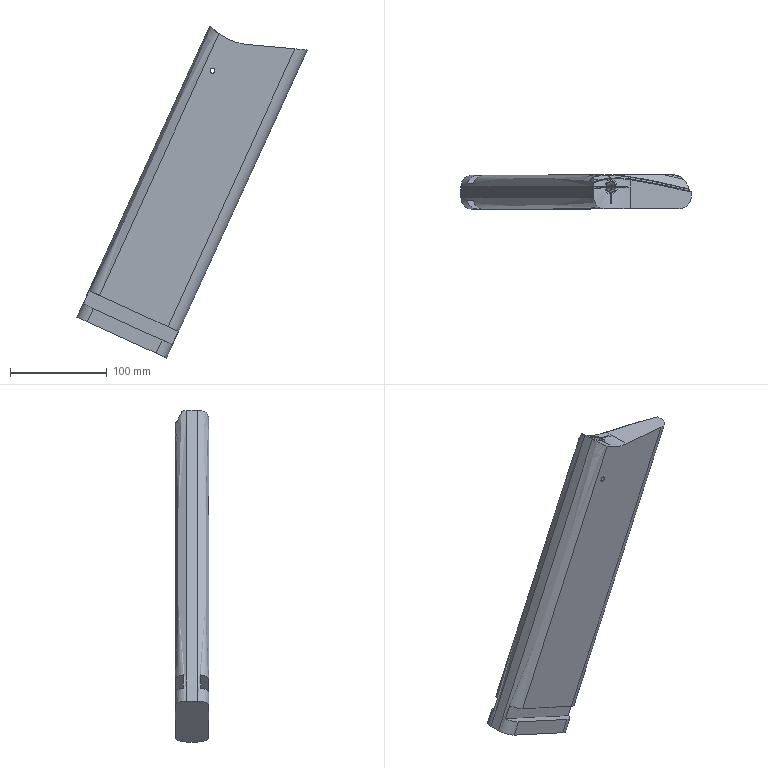Part | STEP file | solid 5 | 1 solid | 145 faces | box 238.099 x 35 x 343.322 mm | volume 1118038 mm3 | plane 63 | other 44 | spline 27 | cylinder 10 | cone 1 | commonest cylinder face diameters 4.02 x3 5 x2 6 x2 24 x2 10 x1